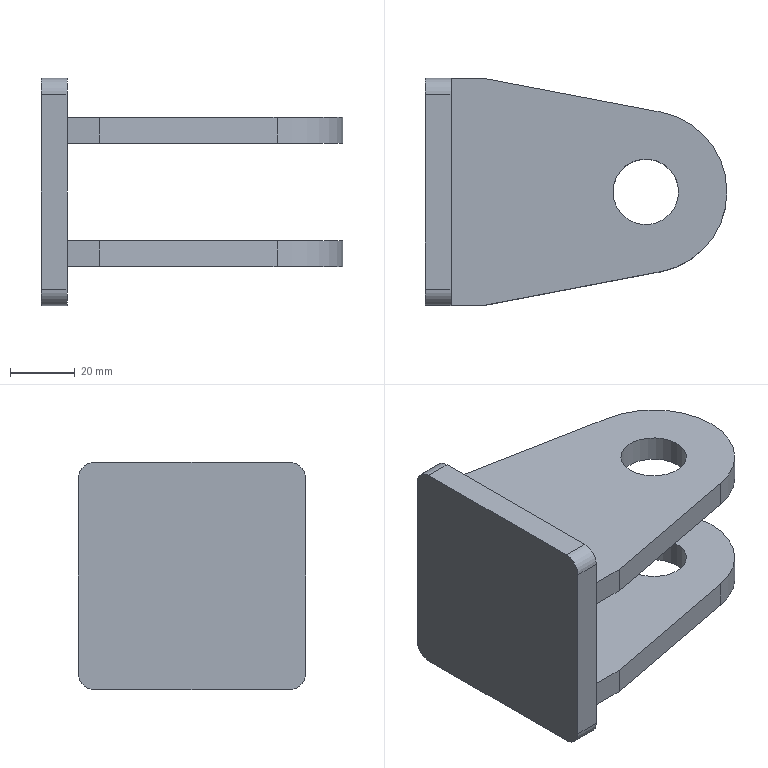Part | STEP file | HL4GZ-1.30.033 (cylinder mounting seat 1 weldment) | 3 solids | 28 faces | box 93 x 70 x 70 mm | volume 109193 mm3 | plane 20 | cylinder 8 | commonest cylinder face diameters 10 x4 20.2 x2 50 x2